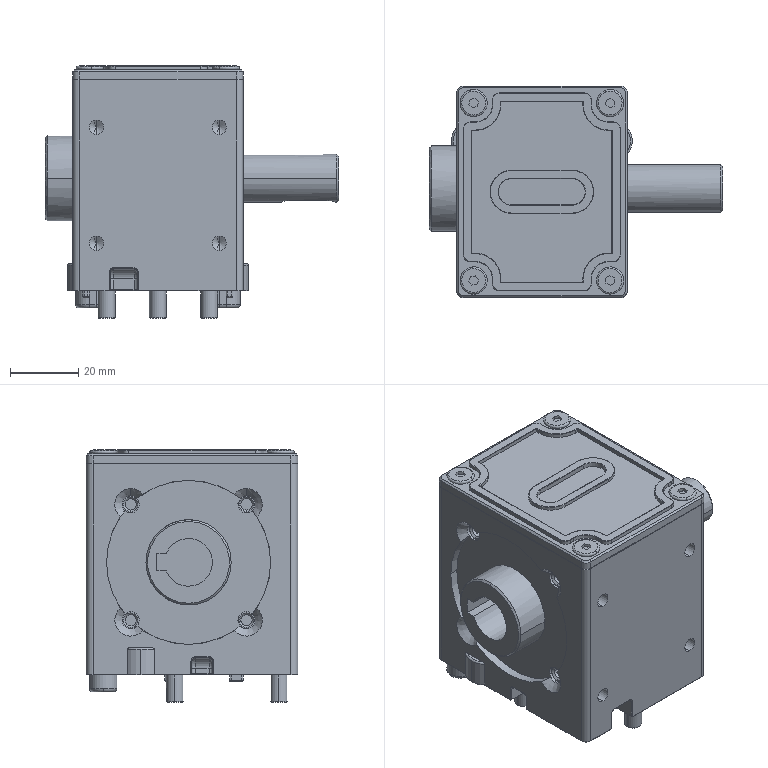Part | SolidWorks | features BaseBody 13, ICE 6, Chamfer 3 | 12 solids | 1016 faces | box 86 x 62 x 74 mm | volume 199634 mm3 | plane 452 | cylinder 309 | cone 179 | torus 56 | sphere 12 | spline 8 | commonest cylinder face diameters 2 x51 5 x33 1 x24 4 x24 0.2 x18 0.6 x16